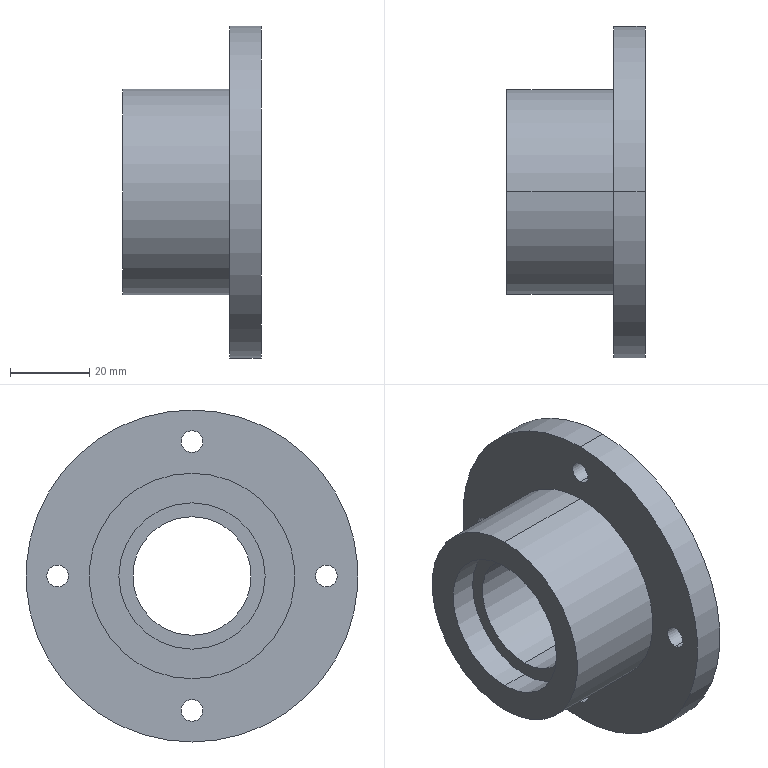Part | STEP file | MT-COMBO-119-S005 | 1 solid | 23 faces | box 35 x 84 x 84 mm | volume 71017 mm3 | cylinder 18 | plane 5 | commonest cylinder face diameters 5.5 x8 37 x4 30 x2 52 x2 84 x2
STEP:
#1=CARTESIAN_POINT('',(27.,-34.,2.75));
#2=VERTEX_POINT('',#1);
#3=CARTESIAN_POINT('',(27.,-34.,-2.75));
#4=VERTEX_POINT('',#3);
#5=CARTESIAN_POINT('',(27.,-34.,0.));
#6=DIRECTION('',(-1.,0.,0.));
#7=DIRECTION('',(0.,0.,1.));
#8=AXIS2_PLACEMENT_3D('',#5,#6,#7);
#9=CIRCLE('',#8,2.75);
#10=EDGE_CURVE('',#2,#4,#9,.T.);
#11=ORIENTED_EDGE('',*,*,#10,.T.);
#12=CARTESIAN_POINT('',(35.,-34.,-2.75));
#13=VERTEX_POINT('',#12);
#14=CARTESIAN_POINT('',(35.,-34.,-2.75));
#15=DIRECTION('',(1.,0.,0.));
#16=VECTOR('',#15,1000.);
#17=LINE('',#14,#16);
#18=EDGE_CURVE('',#4,#13,#17,.T.);
#19=ORIENTED_EDGE('',*,*,#18,.T.);
#20=CARTESIAN_POINT('',(35.,-34.,2.75));
#21=VERTEX_POINT('',#20);
#22=CARTESIAN_POINT('',(35.,-34.,0.));
#23=DIRECTION('',(-1.,0.,0.));
#24=DIRECTION('',(0.,0.,1.));
#25=AXIS2_PLACEMENT_3D('',#22,#23,#24);
#26=CIRCLE('',#25,2.75);
#27=EDGE_CURVE('',#21,#13,#26,.T.);
#28=ORIENTED_EDGE('',*,*,#27,.F.);
#29=CARTESIAN_POINT('',(35.,-34.,2.75));
#30=DIRECTION('',(1.,0.,0.));
#31=VECTOR('',#30,1000.);
#32=LINE('',#29,#31);
#33=EDGE_CURVE('',#2,#21,#32,.T.);
#34=ORIENTED_EDGE('',*,*,#33,.F.);
#35=EDGE_LOOP('',(#11,#19,#28,#34));
#36=FACE_OUTER_BOUND('',#35,.T.);
#37=CARTESIAN_POINT('',(35.,-34.,0.));
#38=DIRECTION('',(1.,0.,0.));
#39=DIRECTION('',(0.,0.,1.));
#40=AXIS2_PLACEMENT_3D('',#37,#38,#39);
#41=CYLINDRICAL_SURFACE('',#40,2.75);
#42=ADVANCED_FACE('',(#36),#41,.F.);
#43=CARTESIAN_POINT('',(27.,0.,-31.25));
#44=VERTEX_POINT('',#43);
#45=CARTESIAN_POINT('',(27.,0.,-36.75));
#46=VERTEX_POINT('',#45);
#47=CARTESIAN_POINT('',(27.,0.,-34.));
#48=DIRECTION('',(-1.,0.,0.));
#49=DIRECTION('',(0.,0.,1.));
#50=AXIS2_PLACEMENT_3D('',#47,#48,#49);
#51=CIRCLE('',#50,2.75);
#52=EDGE_CURVE('',#44,#46,#51,.T.);
#53=ORIENTED_EDGE('',*,*,#52,.T.);
#54=CARTESIAN_POINT('',(35.,0.,-36.75));
#55=VERTEX_POINT('',#54);
#56=CARTESIAN_POINT('',(35.,0.,-36.75));
#57=DIRECTION('',(1.,0.,0.));
#58=VECTOR('',#57,1000.);
#59=LINE('',#56,#58);
#60=EDGE_CURVE('',#46,#55,#59,.T.);
#61=ORIENTED_EDGE('',*,*,#60,.T.);
#62=CARTESIAN_POINT('',(35.,0.,-31.25));
#63=VERTEX_POINT('',#62);
#64=CARTESIAN_POINT('',(35.,0.,-34.));
#65=DIRECTION('',(-1.,0.,0.));
#66=DIRECTION('',(0.,0.,1.));
#67=AXIS2_PLACEMENT_3D('',#64,#65,#66);
#68=CIRCLE('',#67,2.75);
#69=EDGE_CURVE('',#63,#55,#68,.T.);
#70=ORIENTED_EDGE('',*,*,#69,.F.);
#71=CARTESIAN_POINT('',(35.,0.,-31.25));
#72=DIRECTION('',(1.,0.,0.));
#73=VECTOR('',#72,1000.);
#74=LINE('',#71,#73);
#75=EDGE_CURVE('',#44,#63,#74,.T.);
#76=ORIENTED_EDGE('',*,*,#75,.F.);
#77=EDGE_LOOP('',(#53,#61,#70,#76));
#78=FACE_OUTER_BOUND('',#77,.T.);
#79=CARTESIAN_POINT('',(35.,0.,-34.));
#80=DIRECTION('',(1.,0.,0.));
#81=DIRECTION('',(0.,0.,1.));
#82=AXIS2_PLACEMENT_3D('',#79,#80,#81);
#83=CYLINDRICAL_SURFACE('',#82,2.75);
#84=ADVANCED_FACE('',(#78),#83,.F.);
#85=CARTESIAN_POINT('',(27.,34.,2.75));
#86=VERTEX_POINT('',#85);
#87=CARTESIAN_POINT('',(27.,34.,-2.75));
#88=VERTEX_POINT('',#87);
#89=CARTESIAN_POINT('',(27.,34.,0.));
#90=DIRECTION('',(-1.,0.,0.));
#91=DIRECTION('',(0.,0.,1.));
#92=AXIS2_PLACEMENT_3D('',#89,#90,#91);
#93=CIRCLE('',#92,2.75);
#94=EDGE_CURVE('',#86,#88,#93,.T.);
#95=ORIENTED_EDGE('',*,*,#94,.T.);
#96=CARTESIAN_POINT('',(35.,34.,-2.75));
#97=VERTEX_POINT('',#96);
#98=CARTESIAN_POINT('',(35.,34.,-2.75));
#99=DIRECTION('',(1.,0.,0.));
#100=VECTOR('',#99,1000.);
#101=LINE('',#98,#100);
#102=EDGE_CURVE('',#88,#97,#101,.T.);
#103=ORIENTED_EDGE('',*,*,#102,.T.);
#104=CARTESIAN_POINT('',(35.,34.,2.75));
#105=VERTEX_POINT('',#104);
#106=CARTESIAN_POINT('',(35.,34.,0.));
#107=DIRECTION('',(-1.,0.,0.));
#108=DIRECTION('',(0.,0.,1.));
#109=AXIS2_PLACEMENT_3D('',#106,#107,#108);
#110=CIRCLE('',#109,2.75);
#111=EDGE_CURVE('',#105,#97,#110,.T.);
#112=ORIENTED_EDGE('',*,*,#111,.F.);
#113=CARTESIAN_POINT('',(35.,34.,2.75));
#114=DIRECTION('',(1.,0.,0.));
#115=VECTOR('',#114,1000.);
#116=LINE('',#113,#115);
#117=EDGE_CURVE('',#86,#105,#116,.T.);
#118=ORIENTED_EDGE('',*,*,#117,.F.);
#119=EDGE_LOOP('',(#95,#103,#112,#118));
#120=FACE_OUTER_BOUND('',#119,.T.);
#121=CARTESIAN_POINT('',(35.,34.,0.));
#122=DIRECTION('',(1.,0.,0.));
#123=DIRECTION('',(0.,0.,1.));
#124=AXIS2_PLACEMENT_3D('',#121,#122,#123);
#125=CYLINDRICAL_SURFACE('',#124,2.75);
#126=ADVANCED_FACE('',(#120),#125,.F.);
#127=CARTESIAN_POINT('',(27.,0.,36.75));
#128=VERTEX_POINT('',#127);
#129=CARTESIAN_POINT('',(27.,0.,31.25));
#130=VERTEX_POINT('',#129);
#131=CARTESIAN_POINT('',(27.,0.,34.));
#132=DIRECTION('',(-1.,0.,0.));
#133=DIRECTION('',(0.,0.,1.));
#134=AXIS2_PLACEMENT_3D('',#131,#132,#133);
#135=CIRCLE('',#134,2.75);
#136=EDGE_CURVE('',#128,#130,#135,.T.);
#137=ORIENTED_EDGE('',*,*,#136,.T.);
#138=CARTESIAN_POINT('',(35.,0.,31.25));
#139=VERTEX_POINT('',#138);
#140=CARTESIAN_POINT('',(35.,0.,31.25));
#141=DIRECTION('',(1.,0.,0.));
#142=VECTOR('',#141,1000.);
#143=LINE('',#140,#142);
#144=EDGE_CURVE('',#130,#139,#143,.T.);
#145=ORIENTED_EDGE('',*,*,#144,.T.);
#146=CARTESIAN_POINT('',(35.,0.,36.75));
#147=VERTEX_POINT('',#146);
#148=CARTESIAN_POINT('',(35.,0.,34.));
#149=DIRECTION('',(-1.,0.,0.));
#150=DIRECTION('',(0.,0.,1.));
#151=AXIS2_PLACEMENT_3D('',#148,#149,#150);
#152=CIRCLE('',#151,2.75);
#153=EDGE_CURVE('',#147,#139,#152,.T.);
#154=ORIENTED_EDGE('',*,*,#153,.F.);
#155=CARTESIAN_POINT('',(35.,0.,36.75));
#156=DIRECTION('',(1.,0.,0.));
#157=VECTOR('',#156,1000.);
#158=LINE('',#155,#157);
#159=EDGE_CURVE('',#128,#147,#158,.T.);
#160=ORIENTED_EDGE('',*,*,#159,.F.);
#161=EDGE_LOOP('',(#137,#145,#154,#160));
#162=FACE_OUTER_BOUND('',#161,.T.);
#163=CARTESIAN_POINT('',(35.,0.,34.));
#164=DIRECTION('',(1.,0.,0.));
#165=DIRECTION('',(0.,0.,1.));
#166=AXIS2_PLACEMENT_3D('',#163,#164,#165);
#167=CYLINDRICAL_SURFACE('',#166,2.75);
#168=ADVANCED_FACE('',(#162),#167,.F.);
#169=CARTESIAN_POINT('',(35.,0.,-18.5));
#170=VERTEX_POINT('',#169);
#171=CARTESIAN_POINT('',(35.,0.,18.5));
#172=VERTEX_POINT('',#171);
#173=CARTESIAN_POINT('',(35.,0.,0.));
#174=DIRECTION('',(1.,0.,0.));
#175=DIRECTION('',(0.,0.,-1.));
#176=AXIS2_PLACEMENT_3D('',#173,#174,#175);
#177=CIRCLE('',#176,18.5);
#178=EDGE_CURVE('',#170,#172,#177,.T.);
#179=ORIENTED_EDGE('',*,*,#178,.T.);
#180=CARTESIAN_POINT('',(28.,0.,18.5));
#181=VERTEX_POINT('',#180);
#182=CARTESIAN_POINT('',(0.,0.,18.5));
#183=DIRECTION('',(-1.,0.,0.));
#184=VECTOR('',#183,1000.);
#185=LINE('',#182,#184);
#186=EDGE_CURVE('',#172,#181,#185,.T.);
#187=ORIENTED_EDGE('',*,*,#186,.T.);
#188=CARTESIAN_POINT('',(28.,0.,-18.5));
#189=VERTEX_POINT('',#188);
#190=CARTESIAN_POINT('',(28.,0.,0.));
#191=DIRECTION('',(1.,0.,0.));
#192=DIRECTION('',(0.,0.,-1.));
#193=AXIS2_PLACEMENT_3D('',#190,#191,#192);
#194=CIRCLE('',#193,18.5);
#195=EDGE_CURVE('',#189,#181,#194,.T.);
#196=ORIENTED_EDGE('',*,*,#195,.F.);
#197=CARTESIAN_POINT('',(0.,0.,-18.5));
#198=DIRECTION('',(-1.,0.,0.));
#199=VECTOR('',#198,1000.);
#200=LINE('',#197,#199);
#201=EDGE_CURVE('',#170,#189,#200,.T.);
#202=ORIENTED_EDGE('',*,*,#201,.F.);
#203=EDGE_LOOP('',(#179,#187,#196,#202));
#204=FACE_OUTER_BOUND('',#203,.T.);
#205=CARTESIAN_POINT('',(0.,0.,0.));
#206=DIRECTION('',(-1.,0.,0.));
#207=DIRECTION('',(0.,0.,-1.));
#208=AXIS2_PLACEMENT_3D('',#205,#206,#207);
#209=CYLINDRICAL_SURFACE('',#208,18.5);
#210=ADVANCED_FACE('',(#204),#209,.F.);
#211=CARTESIAN_POINT('',(28.,0.,-15.));
#212=VERTEX_POINT('',#211);
#213=CARTESIAN_POINT('',(28.,0.,15.));
#214=VERTEX_POINT('',#213);
#215=CARTESIAN_POINT('',(28.,0.,0.));
#216=DIRECTION('',(1.,0.,0.));
#217=DIRECTION('',(0.,0.,-1.));
#218=AXIS2_PLACEMENT_3D('',#215,#216,#217);
#219=CIRCLE('',#218,15.);
#220=EDGE_CURVE('',#212,#214,#219,.T.);
#221=ORIENTED_EDGE('',*,*,#220,.T.);
#222=CARTESIAN_POINT('',(7.,0.,15.));
#223=VERTEX_POINT('',#222);
#224=CARTESIAN_POINT('',(0.,0.,15.));
#225=DIRECTION('',(-1.,0.,0.));
#226=VECTOR('',#225,1000.);
#227=LINE('',#224,#226);
#228=EDGE_CURVE('',#214,#223,#227,.T.);
#229=ORIENTED_EDGE('',*,*,#228,.T.);
#230=CARTESIAN_POINT('',(7.,0.,-15.));
#231=VERTEX_POINT('',#230);
#232=CARTESIAN_POINT('',(7.,0.,0.));
#233=DIRECTION('',(1.,0.,0.));
#234=DIRECTION('',(0.,0.,-1.));
#235=AXIS2_PLACEMENT_3D('',#232,#233,#234);
#236=CIRCLE('',#235,15.);
#237=EDGE_CURVE('',#231,#223,#236,.T.);
#238=ORIENTED_EDGE('',*,*,#237,.F.);
#239=CARTESIAN_POINT('',(0.,0.,-15.));
#240=DIRECTION('',(-1.,0.,0.));
#241=VECTOR('',#240,1000.);
#242=LINE('',#239,#241);
#243=EDGE_CURVE('',#212,#231,#242,.T.);
#244=ORIENTED_EDGE('',*,*,#243,.F.);
#245=EDGE_LOOP('',(#221,#229,#238,#244));
#246=FACE_OUTER_BOUND('',#245,.T.);
#247=CARTESIAN_POINT('',(0.,0.,0.));
#248=DIRECTION('',(-1.,0.,0.));
#249=DIRECTION('',(0.,0.,-1.));
#250=AXIS2_PLACEMENT_3D('',#247,#248,#249);
#251=CYLINDRICAL_SURFACE('',#250,15.);
#252=ADVANCED_FACE('',(#246),#251,.F.);
#253=CARTESIAN_POINT('',(7.,0.,-18.5));
#254=VERTEX_POINT('',#253);
#255=CARTESIAN_POINT('',(7.,0.,18.5));
#256=VERTEX_POINT('',#255);
#257=CARTESIAN_POINT('',(7.,0.,0.));
#258=DIRECTION('',(1.,0.,0.));
#259=DIRECTION('',(0.,0.,-1.));
#260=AXIS2_PLACEMENT_3D('',#257,#258,#259);
#261=CIRCLE('',#260,18.5);
#262=EDGE_CURVE('',#254,#256,#261,.T.);
#263=ORIENTED_EDGE('',*,*,#262,.T.);
#264=CARTESIAN_POINT('',(0.,0.,18.5));
#265=VERTEX_POINT('',#264);
#266=CARTESIAN_POINT('',(0.,0.,18.5));
#267=DIRECTION('',(-1.,0.,0.));
#268=VECTOR('',#267,1000.);
#269=LINE('',#266,#268);
#270=EDGE_CURVE('',#256,#265,#269,.T.);
#271=ORIENTED_EDGE('',*,*,#270,.T.);
#272=CARTESIAN_POINT('',(0.,0.,-18.5));
#273=VERTEX_POINT('',#272);
#274=CARTESIAN_POINT('',(0.,0.,0.));
#275=DIRECTION('',(1.,0.,0.));
#276=DIRECTION('',(0.,0.,-1.));
#277=AXIS2_PLACEMENT_3D('',#274,#275,#276);
#278=CIRCLE('',#277,18.5);
#279=EDGE_CURVE('',#273,#265,#278,.T.);
#280=ORIENTED_EDGE('',*,*,#279,.F.);
#281=CARTESIAN_POINT('',(0.,0.,-18.5));
#282=DIRECTION('',(-1.,0.,0.));
#283=VECTOR('',#282,1000.);
#284=LINE('',#281,#283);
#285=EDGE_CURVE('',#254,#273,#284,.T.);
#286=ORIENTED_EDGE('',*,*,#285,.F.);
#287=EDGE_LOOP('',(#263,#271,#280,#286));
#288=FACE_OUTER_BOUND('',#287,.T.);
#289=CARTESIAN_POINT('',(0.,0.,0.));
#290=DIRECTION('',(-1.,0.,0.));
#291=DIRECTION('',(0.,0.,-1.));
#292=AXIS2_PLACEMENT_3D('',#289,#290,#291);
#293=CYLINDRICAL_SURFACE('',#292,18.5);
#294=ADVANCED_FACE('',(#288),#293,.F.);
#295=CARTESIAN_POINT('',(27.,0.,26.));
#296=VERTEX_POINT('',#295);
#297=CARTESIAN_POINT('',(27.,0.,-26.));
#298=VERTEX_POINT('',#297);
#299=CARTESIAN_POINT('',(27.,0.,0.));
#300=DIRECTION('',(1.,0.,0.));
#301=DIRECTION('',(0.,0.,-1.));
#302=AXIS2_PLACEMENT_3D('',#299,#300,#301);
#303=CIRCLE('',#302,26.);
#304=EDGE_CURVE('',#296,#298,#303,.T.);
#305=ORIENTED_EDGE('',*,*,#304,.F.);
#306=CARTESIAN_POINT('',(0.,0.,26.));
#307=VERTEX_POINT('',#306);
#308=CARTESIAN_POINT('',(0.,0.,26.));
#309=DIRECTION('',(-1.,0.,0.));
#310=VECTOR('',#309,1000.);
#311=LINE('',#308,#310);
#312=EDGE_CURVE('',#296,#307,#311,.T.);
#313=ORIENTED_EDGE('',*,*,#312,.T.);
#314=CARTESIAN_POINT('',(0.,0.,-26.));
#315=VERTEX_POINT('',#314);
#316=CARTESIAN_POINT('',(0.,0.,0.));
#317=DIRECTION('',(1.,0.,0.));
#318=DIRECTION('',(0.,0.,-1.));
#319=AXIS2_PLACEMENT_3D('',#316,#317,#318);
#320=CIRCLE('',#319,26.);
#321=EDGE_CURVE('',#307,#315,#320,.T.);
#322=ORIENTED_EDGE('',*,*,#321,.T.);
#323=CARTESIAN_POINT('',(0.,0.,-26.));
#324=DIRECTION('',(-1.,0.,0.));
#325=VECTOR('',#324,1000.);
#326=LINE('',#323,#325);
#327=EDGE_CURVE('',#298,#315,#326,.T.);
#328=ORIENTED_EDGE('',*,*,#327,.F.);
#329=EDGE_LOOP('',(#305,#313,#322,#328));
#330=FACE_OUTER_BOUND('',#329,.T.);
#331=CARTESIAN_POINT('',(0.,0.,0.));
#332=DIRECTION('',(-1.,0.,0.));
#333=DIRECTION('',(0.,0.,-1.));
#334=AXIS2_PLACEMENT_3D('',#331,#332,#333);
#335=CYLINDRICAL_SURFACE('',#334,26.);
#336=ADVANCED_FACE('',(#330),#335,.T.);
#337=CARTESIAN_POINT('',(35.,0.,42.));
#338=VERTEX_POINT('',#337);
#339=CARTESIAN_POINT('',(35.,0.,-42.));
#340=VERTEX_POINT('',#339);
#341=CARTESIAN_POINT('',(35.,0.,0.));
#342=DIRECTION('',(1.,0.,0.));
#343=DIRECTION('',(0.,0.,-1.));
#344=AXIS2_PLACEMENT_3D('',#341,#342,#343);
#345=CIRCLE('',#344,42.);
#346=EDGE_CURVE('',#338,#340,#345,.T.);
#347=ORIENTED_EDGE('',*,*,#346,.F.);
#348=CARTESIAN_POINT('',(27.,0.,42.));
#349=VERTEX_POINT('',#348);
#350=CARTESIAN_POINT('',(0.,0.,42.));
#351=DIRECTION('',(-1.,0.,0.));
#352=VECTOR('',#351,1000.);
#353=LINE('',#350,#352);
#354=EDGE_CURVE('',#338,#349,#353,.T.);
#355=ORIENTED_EDGE('',*,*,#354,.T.);
#356=CARTESIAN_POINT('',(27.,0.,-42.));
#357=VERTEX_POINT('',#356);
#358=CARTESIAN_POINT('',(27.,0.,0.));
#359=DIRECTION('',(1.,0.,0.));
#360=DIRECTION('',(0.,0.,-1.));
#361=AXIS2_PLACEMENT_3D('',#358,#359,#360);
#362=CIRCLE('',#361,42.);
#363=EDGE_CURVE('',#349,#357,#362,.T.);
#364=ORIENTED_EDGE('',*,*,#363,.T.);
#365=CARTESIAN_POINT('',(0.,0.,-42.));
#366=DIRECTION('',(-1.,0.,0.));
#367=VECTOR('',#366,1000.);
#368=LINE('',#365,#367);
#369=EDGE_CURVE('',#340,#357,#368,.T.);
#370=ORIENTED_EDGE('',*,*,#369,.F.);
#371=EDGE_LOOP('',(#347,#355,#364,#370));
#372=FACE_OUTER_BOUND('',#371,.T.);
#373=CARTESIAN_POINT('',(0.,0.,0.));
#374=DIRECTION('',(-1.,0.,0.));
#375=DIRECTION('',(0.,0.,-1.));
#376=AXIS2_PLACEMENT_3D('',#373,#374,#375);
#377=CYLINDRICAL_SURFACE('',#376,42.);
#378=ADVANCED_FACE('',(#372),#377,.T.);
#379=ORIENTED_EDGE('',*,*,#27,.T.);
#380=CARTESIAN_POINT('',(35.,-34.,0.));
#381=DIRECTION('',(-1.,0.,0.));
#382=DIRECTION('',(0.,0.,1.));
#383=AXIS2_PLACEMENT_3D('',#380,#381,#382);
#384=CIRCLE('',#383,2.75);
#385=EDGE_CURVE('',#13,#21,#384,.T.);
#386=ORIENTED_EDGE('',*,*,#385,.T.);
#387=EDGE_LOOP('',(#379,#386));
#388=FACE_BOUND('',#387,.T.);
#389=ORIENTED_EDGE('',*,*,#69,.T.);
#390=CARTESIAN_POINT('',(35.,0.,-34.));
#391=DIRECTION('',(-1.,0.,0.));
#392=DIRECTION('',(0.,0.,1.));
#393=AXIS2_PLACEMENT_3D('',#390,#391,#392);
#394=CIRCLE('',#393,2.75);
#395=EDGE_CURVE('',#55,#63,#394,.T.);
#396=ORIENTED_EDGE('',*,*,#395,.T.);
#397=EDGE_LOOP('',(#389,#396));
#398=FACE_BOUND('',#397,.T.);
#399=ORIENTED_EDGE('',*,*,#111,.T.);
#400=CARTESIAN_POINT('',(35.,34.,0.));
#401=DIRECTION('',(-1.,0.,0.));
#402=DIRECTION('',(0.,0.,1.));
#403=AXIS2_PLACEMENT_3D('',#400,#401,#402);
#404=CIRCLE('',#403,2.75);
#405=EDGE_CURVE('',#97,#105,#404,.T.);
#406=ORIENTED_EDGE('',*,*,#405,.T.);
#407=EDGE_LOOP('',(#399,#406));
#408=FACE_BOUND('',#407,.T.);
#409=ORIENTED_EDGE('',*,*,#153,.T.);
#410=CARTESIAN_POINT('',(35.,0.,34.));
#411=DIRECTION('',(-1.,0.,0.));
#412=DIRECTION('',(0.,0.,1.));
#413=AXIS2_PLACEMENT_3D('',#410,#411,#412);
#414=CIRCLE('',#413,2.75);
#415=EDGE_CURVE('',#139,#147,#414,.T.);
#416=ORIENTED_EDGE('',*,*,#415,.T.);
#417=EDGE_LOOP('',(#409,#416));
#418=FACE_BOUND('',#417,.T.);
#419=ORIENTED_EDGE('',*,*,#178,.F.);
#420=CARTESIAN_POINT('',(35.,0.,0.));
#421=DIRECTION('',(1.,0.,0.));
#422=DIRECTION('',(0.,0.,-1.));
#423=AXIS2_PLACEMENT_3D('',#420,#421,#422);
#424=CIRCLE('',#423,18.5);
#425=EDGE_CURVE('',#172,#170,#424,.T.);
#426=ORIENTED_EDGE('',*,*,#425,.F.);
#427=EDGE_LOOP('',(#419,#426));
#428=FACE_BOUND('',#427,.T.);
#429=CARTESIAN_POINT('',(35.,0.,0.));
#430=DIRECTION('',(1.,0.,0.));
#431=DIRECTION('',(0.,0.,-1.));
#432=AXIS2_PLACEMENT_3D('',#429,#430,#431);
#433=CIRCLE('',#432,42.);
#434=EDGE_CURVE('',#340,#338,#433,.T.);
#435=ORIENTED_EDGE('',*,*,#434,.T.);
#436=ORIENTED_EDGE('',*,*,#346,.T.);
#437=EDGE_LOOP('',(#435,#436));
#438=FACE_OUTER_BOUND('',#437,.T.);
#439=CARTESIAN_POINT('',(35.,0.,0.));
#440=DIRECTION('',(-1.,0.,0.));
#441=DIRECTION('',(0.,0.,-1.));
#442=AXIS2_PLACEMENT_3D('',#439,#440,#441);
#443=PLANE('',#442);
#444=ADVANCED_FACE('',(#388,#398,#408,#418,#428,#438),#443,.F.);
#445=ORIENTED_EDGE('',*,*,#354,.F.);
#446=ORIENTED_EDGE('',*,*,#434,.F.);
#447=ORIENTED_EDGE('',*,*,#369,.T.);
#448=CARTESIAN_POINT('',(27.,0.,0.));
#449=DIRECTION('',(1.,0.,0.));
#450=DIRECTION('',(0.,0.,-1.));
#451=AXIS2_PLACEMENT_3D('',#448,#449,#450);
#452=CIRCLE('',#451,42.);
#453=EDGE_CURVE('',#357,#349,#452,.T.);
#454=ORIENTED_EDGE('',*,*,#453,.T.);
#455=EDGE_LOOP('',(#445,#446,#447,#454));
#456=FACE_OUTER_BOUND('',#455,.T.);
#457=CARTESIAN_POINT('',(0.,0.,0.));
#458=DIRECTION('',(-1.,0.,0.));
#459=DIRECTION('',(0.,0.,-1.));
#460=AXIS2_PLACEMENT_3D('',#457,#458,#459);
#461=CYLINDRICAL_SURFACE('',#460,42.);
#462=ADVANCED_FACE('',(#456),#461,.T.);
#463=ORIENTED_EDGE('',*,*,#10,.F.);
#464=CARTESIAN_POINT('',(27.,-34.,0.));
#465=DIRECTION('',(-1.,0.,0.));
#466=DIRECTION('',(0.,0.,1.));
#467=AXIS2_PLACEMENT_3D('',#464,#465,#466);
#468=CIRCLE('',#467,2.75);
#469=EDGE_CURVE('',#4,#2,#468,.T.);
#470=ORIENTED_EDGE('',*,*,#469,.F.);
#471=EDGE_LOOP('',(#463,#470));
#472=FACE_BOUND('',#471,.T.);
#473=ORIENTED_EDGE('',*,*,#52,.F.);
#474=CARTESIAN_POINT('',(27.,0.,-34.));
#475=DIRECTION('',(-1.,0.,0.));
#476=DIRECTION('',(0.,0.,1.));
#477=AXIS2_PLACEMENT_3D('',#474,#475,#476);
#478=CIRCLE('',#477,2.75);
#479=EDGE_CURVE('',#46,#44,#478,.T.);
#480=ORIENTED_EDGE('',*,*,#479,.F.);
#481=EDGE_LOOP('',(#473,#480));
#482=FACE_BOUND('',#481,.T.);
#483=ORIENTED_EDGE('',*,*,#94,.F.);
#484=CARTESIAN_POINT('',(27.,34.,0.));
#485=DIRECTION('',(-1.,0.,0.));
#486=DIRECTION('',(0.,0.,1.));
#487=AXIS2_PLACEMENT_3D('',#484,#485,#486);
#488=CIRCLE('',#487,2.75);
#489=EDGE_CURVE('',#88,#86,#488,.T.);
#490=ORIENTED_EDGE('',*,*,#489,.F.);
#491=EDGE_LOOP('',(#483,#490));
#492=FACE_BOUND('',#491,.T.);
#493=ORIENTED_EDGE('',*,*,#136,.F.);
#494=CARTESIAN_POINT('',(27.,0.,34.));
#495=DIRECTION('',(-1.,0.,0.));
#496=DIRECTION('',(0.,0.,1.));
#497=AXIS2_PLACEMENT_3D('',#494,#495,#496);
#498=CIRCLE('',#497,2.75);
#499=EDGE_CURVE('',#130,#128,#498,.T.);
#500=ORIENTED_EDGE('',*,*,#499,.F.);
#501=EDGE_LOOP('',(#493,#500));
#502=FACE_BOUND('',#501,.T.);
#503=CARTESIAN_POINT('',(27.,0.,0.));
#504=DIRECTION('',(1.,0.,0.));
#505=DIRECTION('',(0.,0.,-1.));
#506=AXIS2_PLACEMENT_3D('',#503,#504,#505);
#507=CIRCLE('',#506,26.);
#508=EDGE_CURVE('',#298,#296,#507,.T.);
#509=ORIENTED_EDGE('',*,*,#508,.T.);
#510=ORIENTED_EDGE('',*,*,#304,.T.);
#511=EDGE_LOOP('',(#509,#510));
#512=FACE_BOUND('',#511,.T.);
#513=ORIENTED_EDGE('',*,*,#453,.F.);
#514=ORIENTED_EDGE('',*,*,#363,.F.);
#515=EDGE_LOOP('',(#513,#514));
#516=FACE_OUTER_BOUND('',#515,.T.);
#517=CARTESIAN_POINT('',(27.,42.,0.));
#518=DIRECTION('',(1.,0.,0.));
#519=DIRECTION('',(0.,0.,1.));
#520=AXIS2_PLACEMENT_3D('',#517,#518,#519);
#521=PLANE('',#520);
#522=ADVANCED_FACE('',(#472,#482,#492,#502,#512,#516),#521,.F.);
#523=ORIENTED_EDGE('',*,*,#312,.F.);
#524=ORIENTED_EDGE('',*,*,#508,.F.);
#525=ORIENTED_EDGE('',*,*,#327,.T.);
#526=CARTESIAN_POINT('',(0.,0.,0.));
#527=DIRECTION('',(1.,0.,0.));
#528=DIRECTION('',(0.,0.,-1.));
#529=AXIS2_PLACEMENT_3D('',#526,#527,#528);
#530=CIRCLE('',#529,26.);
#531=EDGE_CURVE('',#315,#307,#530,.T.);
#532=ORIENTED_EDGE('',*,*,#531,.T.);
#533=EDGE_LOOP('',(#523,#524,#525,#532));
#534=FACE_OUTER_BOUND('',#533,.T.);
#535=CARTESIAN_POINT('',(0.,0.,0.));
#536=DIRECTION('',(-1.,0.,0.));
#537=DIRECTION('',(0.,0.,-1.));
#538=AXIS2_PLACEMENT_3D('',#535,#536,#537);
#539=CYLINDRICAL_SURFACE('',#538,26.);
#540=ADVANCED_FACE('',(#534),#539,.T.);
#541=ORIENTED_EDGE('',*,*,#279,.T.);
#542=CARTESIAN_POINT('',(0.,0.,0.));
#543=DIRECTION('',(1.,0.,0.));
#544=DIRECTION('',(0.,0.,-1.));
#545=AXIS2_PLACEMENT_3D('',#542,#543,#544);
#546=CIRCLE('',#545,18.5);
#547=EDGE_CURVE('',#265,#273,#546,.T.);
#548=ORIENTED_EDGE('',*,*,#547,.T.);
#549=EDGE_LOOP('',(#541,#548));
#550=FACE_BOUND('',#549,.T.);
#551=ORIENTED_EDGE('',*,*,#531,.F.);
#552=ORIENTED_EDGE('',*,*,#321,.F.);
#553=EDGE_LOOP('',(#551,#552));
#554=FACE_OUTER_BOUND('',#553,.T.);
#555=CARTESIAN_POINT('',(0.,26.,0.));
#556=DIRECTION('',(1.,0.,0.));
#557=DIRECTION('',(0.,0.,1.));
#558=AXIS2_PLACEMENT_3D('',#555,#556,#557);
#559=PLANE('',#558);
#560=ADVANCED_FACE('',(#550,#554),#559,.F.);
#561=ORIENTED_EDGE('',*,*,#270,.F.);
#562=CARTESIAN_POINT('',(7.,0.,0.));
#563=DIRECTION('',(1.,0.,0.));
#564=DIRECTION('',(0.,0.,-1.));
#565=AXIS2_PLACEMENT_3D('',#562,#563,#564);
#566=CIRCLE('',#565,18.5);
#567=EDGE_CURVE('',#256,#254,#566,.T.);
#568=ORIENTED_EDGE('',*,*,#567,.T.);
#569=ORIENTED_EDGE('',*,*,#285,.T.);
#570=ORIENTED_EDGE('',*,*,#547,.F.);
#571=EDGE_LOOP('',(#561,#568,#569,#570));
#572=FACE_OUTER_BOUND('',#571,.T.);
#573=CARTESIAN_POINT('',(0.,0.,0.));
#574=DIRECTION('',(-1.,0.,0.));
#575=DIRECTION('',(0.,0.,-1.));
#576=AXIS2_PLACEMENT_3D('',#573,#574,#575);
#577=CYLINDRICAL_SURFACE('',#576,18.5);
#578=ADVANCED_FACE('',(#572),#577,.F.);
#579=ORIENTED_EDGE('',*,*,#262,.F.);
#580=ORIENTED_EDGE('',*,*,#567,.F.);
#581=EDGE_LOOP('',(#579,#580));
#582=FACE_OUTER_BOUND('',#581,.T.);
#583=ORIENTED_EDGE('',*,*,#237,.T.);
#584=CARTESIAN_POINT('',(7.,0.,0.));
#585=DIRECTION('',(1.,0.,0.));
#586=DIRECTION('',(0.,0.,-1.));
#587=AXIS2_PLACEMENT_3D('',#584,#585,#586);
#588=CIRCLE('',#587,15.);
#589=EDGE_CURVE('',#223,#231,#588,.T.);
#590=ORIENTED_EDGE('',*,*,#589,.T.);
#591=EDGE_LOOP('',(#583,#590));
#592=FACE_BOUND('',#591,.T.);
#593=CARTESIAN_POINT('',(7.,0.,18.5));
#594=DIRECTION('',(-1.,0.,0.));
#595=DIRECTION('',(0.,0.,-1.));
#596=AXIS2_PLACEMENT_3D('',#593,#594,#595);
#597=PLANE('',#596);
#598=ADVANCED_FACE('',(#582,#592),#597,.T.);
#599=ORIENTED_EDGE('',*,*,#228,.F.);
#600=CARTESIAN_POINT('',(28.,0.,0.));
#601=DIRECTION('',(1.,0.,0.));
#602=DIRECTION('',(0.,0.,-1.));
#603=AXIS2_PLACEMENT_3D('',#600,#601,#602);
#604=CIRCLE('',#603,15.);
#605=EDGE_CURVE('',#214,#212,#604,.T.);
#606=ORIENTED_EDGE('',*,*,#605,.T.);
#607=ORIENTED_EDGE('',*,*,#243,.T.);
#608=ORIENTED_EDGE('',*,*,#589,.F.);
#609=EDGE_LOOP('',(#599,#606,#607,#608));
#610=FACE_OUTER_BOUND('',#609,.T.);
#611=CARTESIAN_POINT('',(0.,0.,0.));
#612=DIRECTION('',(-1.,0.,0.));
#613=DIRECTION('',(0.,0.,-1.));
#614=AXIS2_PLACEMENT_3D('',#611,#612,#613);
#615=CYLINDRICAL_SURFACE('',#614,15.);
#616=ADVANCED_FACE('',(#610),#615,.F.);
#617=ORIENTED_EDGE('',*,*,#220,.F.);
#618=ORIENTED_EDGE('',*,*,#605,.F.);
#619=EDGE_LOOP('',(#617,#618));
#620=FACE_BOUND('',#619,.T.);
#621=ORIENTED_EDGE('',*,*,#195,.T.);
#622=CARTESIAN_POINT('',(28.,0.,0.));
#623=DIRECTION('',(1.,0.,0.));
#624=DIRECTION('',(0.,0.,-1.));
#625=AXIS2_PLACEMENT_3D('',#622,#623,#624);
#626=CIRCLE('',#625,18.5);
#627=EDGE_CURVE('',#181,#189,#626,.T.);
#628=ORIENTED_EDGE('',*,*,#627,.T.);
#629=EDGE_LOOP('',(#621,#628));
#630=FACE_OUTER_BOUND('',#629,.T.);
#631=CARTESIAN_POINT('',(28.,0.,15.));
#632=DIRECTION('',(1.,0.,0.));
#633=DIRECTION('',(0.,0.,1.));
#634=AXIS2_PLACEMENT_3D('',#631,#632,#633);
#635=PLANE('',#634);
#636=ADVANCED_FACE('',(#620,#630),#635,.T.);
#637=ORIENTED_EDGE('',*,*,#186,.F.);
#638=ORIENTED_EDGE('',*,*,#425,.T.);
#639=ORIENTED_EDGE('',*,*,#201,.T.);
#640=ORIENTED_EDGE('',*,*,#627,.F.);
#641=EDGE_LOOP('',(#637,#638,#639,#640));
#642=FACE_OUTER_BOUND('',#641,.T.);
#643=CARTESIAN_POINT('',(0.,0.,0.));
#644=DIRECTION('',(-1.,0.,0.));
#645=DIRECTION('',(0.,0.,-1.));
#646=AXIS2_PLACEMENT_3D('',#643,#644,#645);
#647=CYLINDRICAL_SURFACE('',#646,18.5);
#648=ADVANCED_FACE('',(#642),#647,.F.);
#649=ORIENTED_EDGE('',*,*,#144,.F.);
#650=ORIENTED_EDGE('',*,*,#499,.T.);
#651=ORIENTED_EDGE('',*,*,#159,.T.);
#652=ORIENTED_EDGE('',*,*,#415,.F.);
#653=EDGE_LOOP('',(#649,#650,#651,#652));
#654=FACE_OUTER_BOUND('',#653,.T.);
#655=CARTESIAN_POINT('',(35.,0.,34.));
#656=DIRECTION('',(1.,0.,0.));
#657=DIRECTION('',(0.,0.,1.));
#658=AXIS2_PLACEMENT_3D('',#655,#656,#657);
#659=CYLINDRICAL_SURFACE('',#658,2.75);
#660=ADVANCED_FACE('',(#654),#659,.F.);
#661=ORIENTED_EDGE('',*,*,#102,.F.);
#662=ORIENTED_EDGE('',*,*,#489,.T.);
#663=ORIENTED_EDGE('',*,*,#117,.T.);
#664=ORIENTED_EDGE('',*,*,#405,.F.);
#665=EDGE_LOOP('',(#661,#662,#663,#664));
#666=FACE_OUTER_BOUND('',#665,.T.);
#667=CARTESIAN_POINT('',(35.,34.,0.));
#668=DIRECTION('',(1.,0.,0.));
#669=DIRECTION('',(0.,0.,1.));
#670=AXIS2_PLACEMENT_3D('',#667,#668,#669);
#671=CYLINDRICAL_SURFACE('',#670,2.75);
#672=ADVANCED_FACE('',(#666),#671,.F.);
#673=ORIENTED_EDGE('',*,*,#60,.F.);
#674=ORIENTED_EDGE('',*,*,#479,.T.);
#675=ORIENTED_EDGE('',*,*,#75,.T.);
#676=ORIENTED_EDGE('',*,*,#395,.F.);
#677=EDGE_LOOP('',(#673,#674,#675,#676));
#678=FACE_OUTER_BOUND('',#677,.T.);
#679=CARTESIAN_POINT('',(35.,0.,-34.));
#680=DIRECTION('',(1.,0.,0.));
#681=DIRECTION('',(0.,0.,1.));
#682=AXIS2_PLACEMENT_3D('',#679,#680,#681);
#683=CYLINDRICAL_SURFACE('',#682,2.75);
#684=ADVANCED_FACE('',(#678),#683,.F.);
#685=ORIENTED_EDGE('',*,*,#18,.F.);
#686=ORIENTED_EDGE('',*,*,#469,.T.);
#687=ORIENTED_EDGE('',*,*,#33,.T.);
#688=ORIENTED_EDGE('',*,*,#385,.F.);
#689=EDGE_LOOP('',(#685,#686,#687,#688));
#690=FACE_OUTER_BOUND('',#689,.T.);
#691=CARTESIAN_POINT('',(35.,-34.,0.));
#692=DIRECTION('',(1.,0.,0.));
#693=DIRECTION('',(0.,0.,1.));
#694=AXIS2_PLACEMENT_3D('',#691,#692,#693);
#695=CYLINDRICAL_SURFACE('',#694,2.75);
#696=ADVANCED_FACE('',(#690),#695,.F.);
#697=CLOSED_SHELL('',(#42,#84,#126,#168,#210,#252,#294,#336,#378,#444,#462,#522,#540,#560,#578,#598,#616,#636,#648,#660,#672,#684,#696));
#698=MANIFOLD_SOLID_BREP('',#697);
#699=CARTESIAN_POINT('',(0.,0.,0.));
#700=DIRECTION('',(0.,0.,1.));
#701=DIRECTION('',(1.,0.,0.));
#702=AXIS2_PLACEMENT_3D('',#699,#700,#701);
#703=(LENGTH_UNIT()NAMED_UNIT(*)SI_UNIT(.MILLI.,.METRE.));
#704=UNCERTAINTY_MEASURE_WITH_UNIT(LENGTH_MEASURE(0.00001),#703,'','');
#705=(NAMED_UNIT(*)PLANE_ANGLE_UNIT()SI_UNIT($,.RADIAN.));
#706=(NAMED_UNIT(*)SI_UNIT($,.STERADIAN.)SOLID_ANGLE_UNIT());
#707=(GEOMETRIC_REPRESENTATION_CONTEXT(3)GLOBAL_UNCERTAINTY_ASSIGNED_CONTEXT((#704))GLOBAL_UNIT_ASSIGNED_CONTEXT((#703,#705,#706))REPRESENTATION_CONTEXT('',''));
#708=ADVANCED_BREP_SHAPE_REPRESENTATION('',(#698,#702),#707);